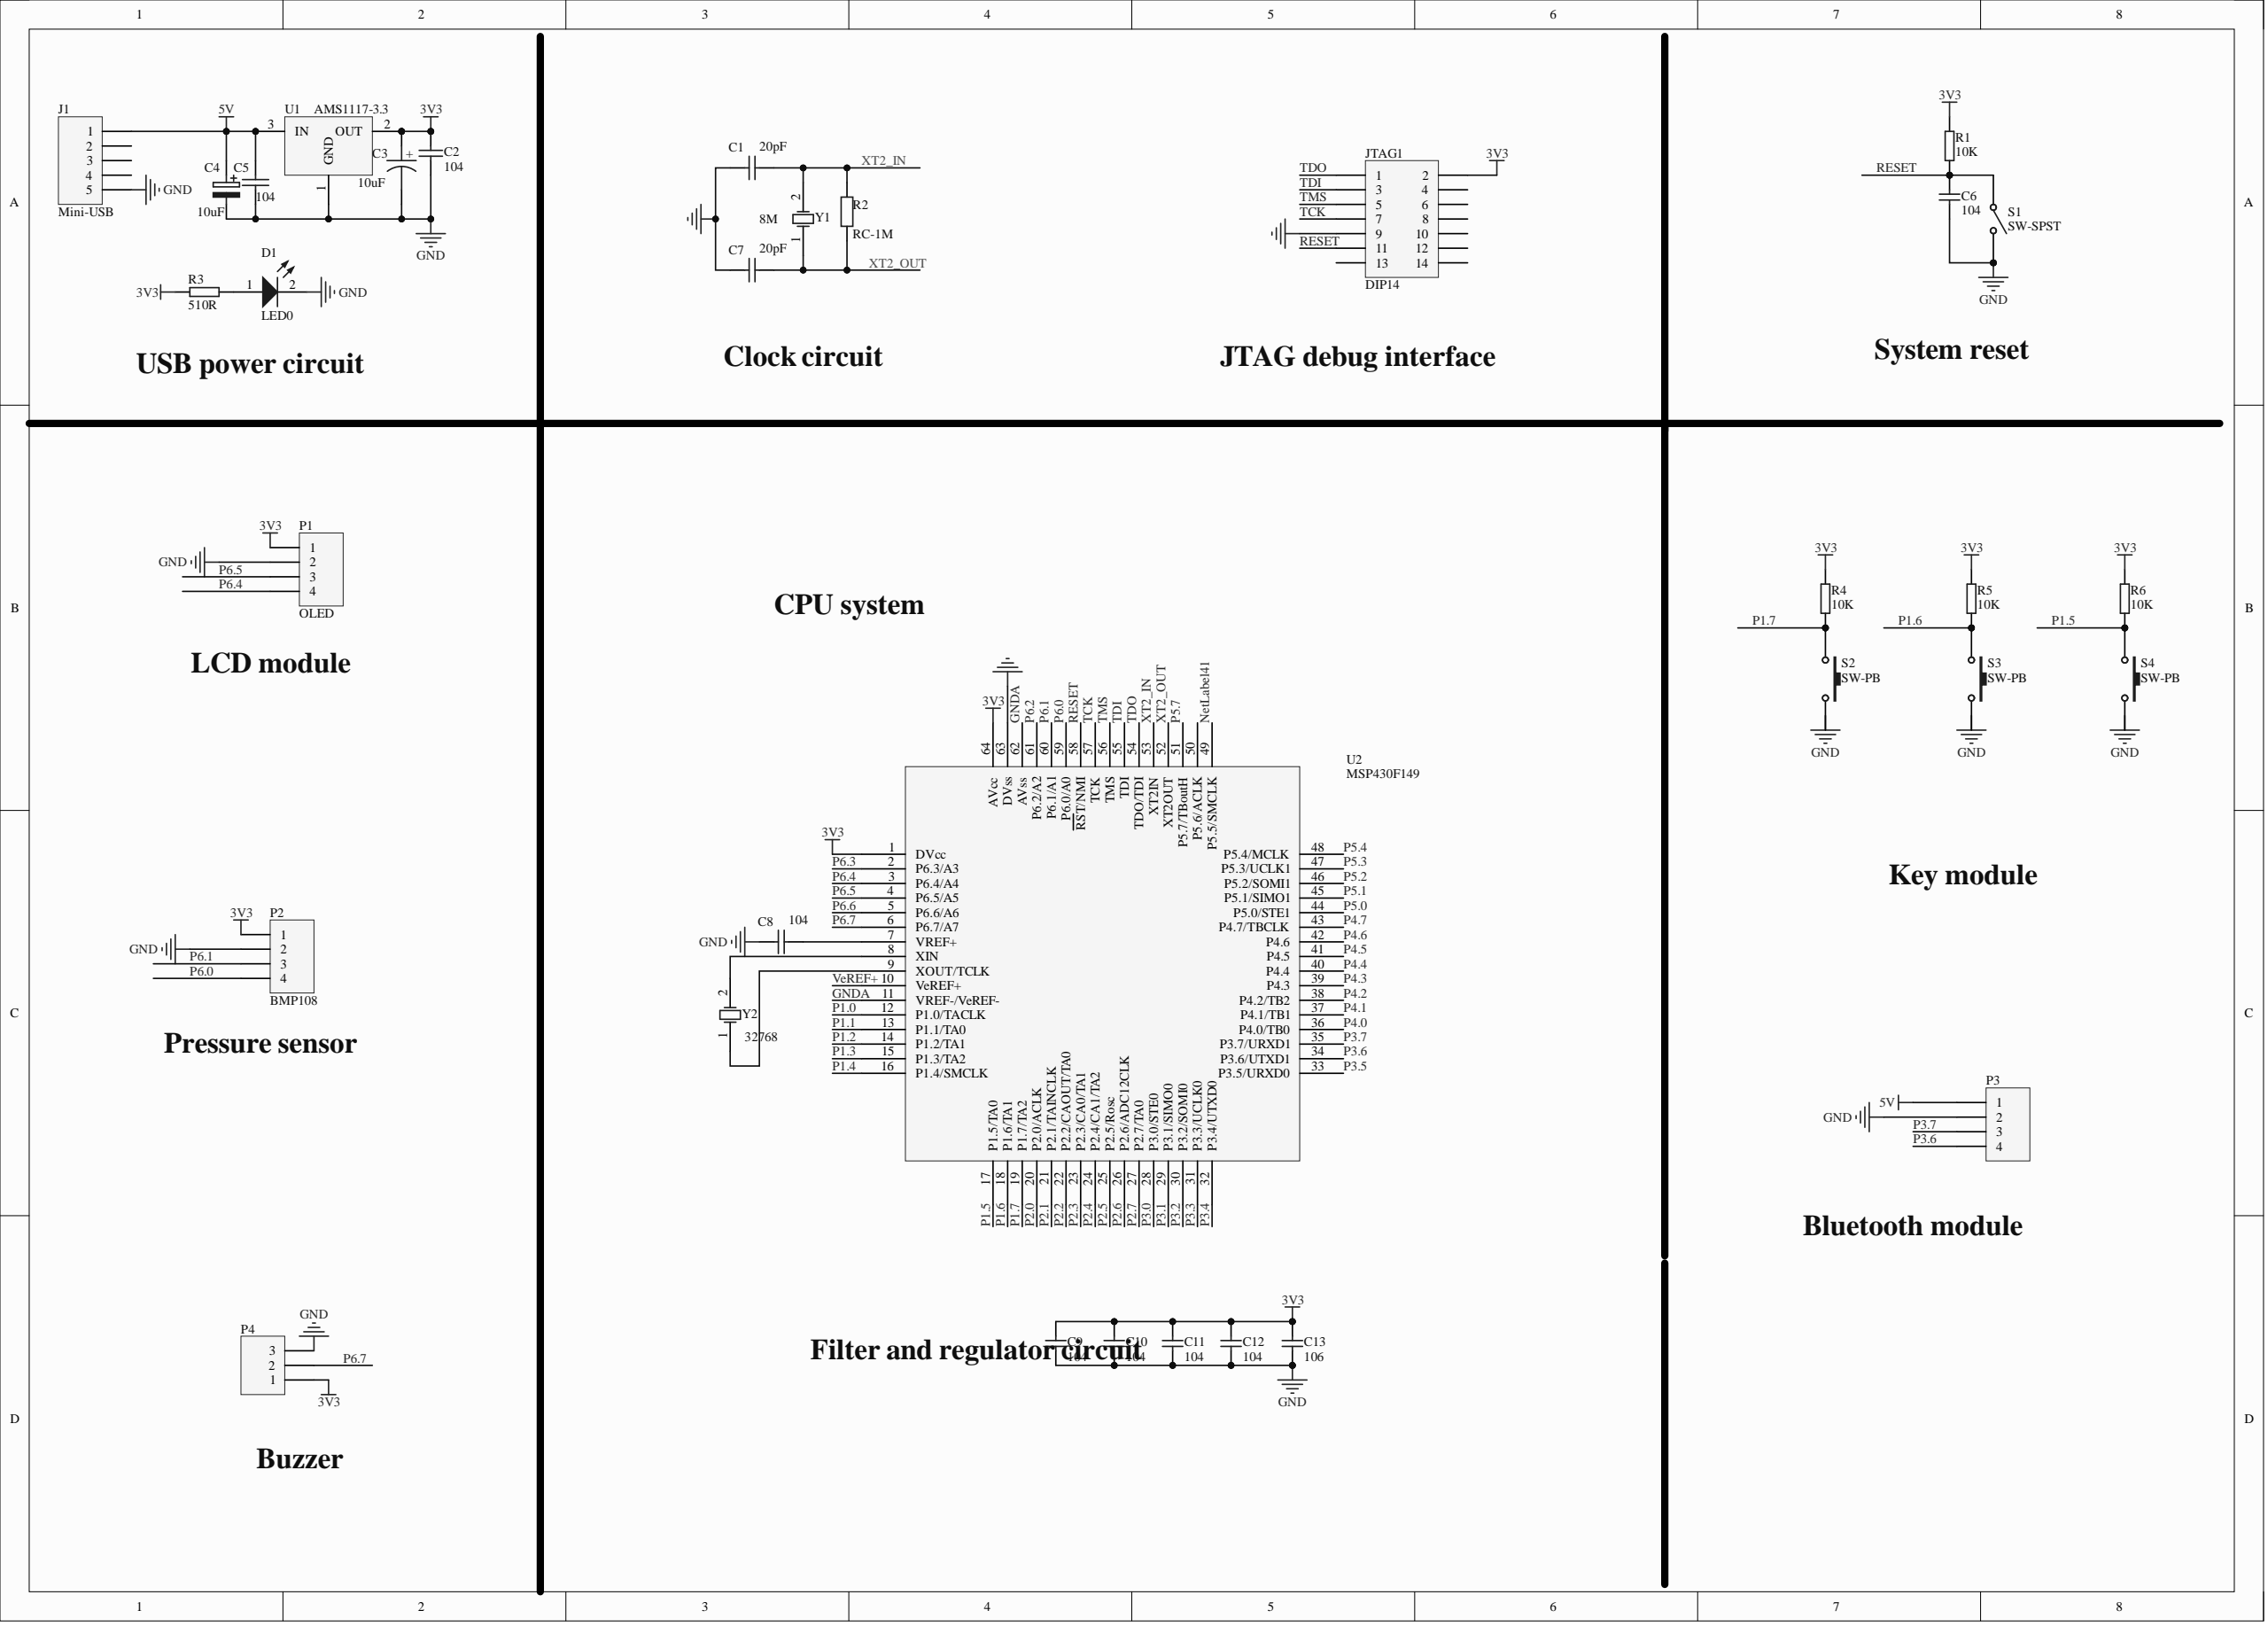Circuit board | Altium Designer | 34 parts | 25 nets
Bill of materials:
Comment,Description,Designator,Footprint,LibRef,Quantity
"S0805-20P","Capacitor","C1, C7, C8","0805C","Cap","3"
"104","Capacitor","C2, C5, C6, C9, C10, C11, C12","0603C","Cap, CAP1","7"
"10uF","Capacitor","C3","贴片电容","CAPACITOR POL","1"
"10uF","","C4","0805C","ELECTRO2","1"
"106","Capacitor","C13","0805C","CAP1","1"
"LED0","Typical INFRARED GaAs LED","D1","LED0603-RD","LED0","1"
"Mini-USB","Header, 5-Pin","J1","USB-MINI-A","Header 5","1"
"DIP14","Connectors","JTAG1","HDR2X7","DIP14","1"
"OLED","Header, 4-Pin, Right Angle","P1","HDR1X4H","Header 4H","1"
"BMP108","Header, 4-Pin, Right Angle","P2","HDR1X4H","Header 4H","1"
"Bluetooth module","Header, 4-Pin","P3","HDR1X4","Header 4","1"
"Buzzer","Header, 3-Pin","P4","HDR1X3","Header 3","1"
"10K","","R1, R4, R5, R6","0603R","R","4"
"RC-1M","Resistor","R2","0805R","Res2","1"
"510R","","R3","0603R","R","1"
"SW-SPST","Single-Pole, Single-Throw Switch","S1","SPST-2","SW-SPST","1"
"SW-PB","Switch","S2, S3, S4","SPST-2","SW-PB","3"
"AMS1117-3.3","","U1","AMS1117-3.3","LT1085CM-3.3","1"
"MSP430F149","MCU","U2","MSP430F149","MSP430F149","1"
"8M","Crystal Oscillator","Y1","XTAL-SMD-NX3215SA-32.768K-STD-MUS-2","XTAL","1"
"32768","Crystal Oscillator","Y2","XTAL-SMD-NX3215SA-32.768K-STD-MUS-2","XTAL","1"
Netlist (Protel format):
[
C1
0805C
S0805-20P



]
[
C2
0603C
104



]
[
C3
贴片电容
10uF



]
[
C4
0805C
10uF



]
[
C5
0603C
104



]
[
C6
0603C
104



]
[
C7
0805C
S0805-20P



]
[
C8
0805C
S0805-20P



]
[
C9
0603C
104



]
[
C10
0603C
104



]
[
C11
0603C
104



]
[
C12
0603C
104



]
[
C13
0805C
106



]
[
D1
LED0603-RD
LED0



]
[
J1
USB-MINI-A
Mini-USB



]
[
JTAG1
HDR2X7
DIP14



]
[
P1
HDR1X4H
OLED



]
[
P2
HDR1X4H
BMP108



]
[
P3
HDR1X4
Bluetooth module



]
[
P4
HDR1X3
Buzzer



]
[
R1
0603R
10K



]
[
R2
0805R
RC-1M



]
[
R3
0603R
510R



]
[
R4
0603R
10K



]
[
R5
0603R
10K



]
[
R6
0603R
10K



]
[
S1
SPST-2
SW-SPST



]
[
S2
SPST-2
SW-PB



]
[
S3
SPST-2
SW-PB



]
[
S4
SPST-2
SW-PB



]
[
U1
AMS1117-3.3
AMS1117-3.3



]
[
U2
MSP430F149
MSP430F149



]
[
Y1
XTAL-SMD-NX3215SA-32.768K-STD-MUS-2
8M



]
[
Y2
XTAL-SMD-NX3215SA-32.768K-STD-MUS-2
32768



]
(
XT2_OUT
C7-2
R2-1
U2-52
Y1-1
)
(
XT2_IN
C1-2
R2-2
U2-53
Y1-2
)
(
TMS
JTAG1-5
U2-56
)
(
TDO
JTAG1-1
U2-54
)
(
TDI
JTAG1-3
U2-55
)
(
TCK
JTAG1-7
U2-57
)
(
RESET
C6-1
JTAG1-11
R1-1
S1-1
U2-58
)
(
P6.7
P4-2
U2-6
)
(
P6.5
P1-3
U2-4
)
(
P6.4
P1-4
U2-3
)
(
P6.1
P2-3
U2-60
)
(
P6.0
P2-4
U2-59
)
(
P3.7
P3-3
U2-35
)
(
P3.6
P3-4
U2-34
)
(
P1.7
R4-1
S2-1
U2-19
)
(
P1.6
R5-1
S3-1
U2-18
)
(
P1.5
R6-1
S4-1
U2-17
)
(
NetU2_9
U2-9
Y2-1
)
(
NetU2_8
U2-8
Y2-2
)
(
NetD1_1
D1-1
R3-1
)
(
NetC8_2
C8-2
U2-7
)
(
GNDA
U2-11
U2-62
)
(
GND
C1-1
C2-2
C3-2
C4-2
C5-2
C6-2
C7-1
C8-1
C9-2
C10-2
C11-2
C12-2
C13-2
D1-2
J1-5
JTAG1-9
P1-2
P2-2
P3-2
P4-3
S1-2
U1-1
U2-63
)
(
5V
C4-1
C5-1
J1-1
P3-1
U1-3
)
(
3V3
C2-1
C3-1
C9-1
C10-1
C11-1
C12-1
C13-1
JTAG1-2
P1-1
P2-1
P4-1
R1-2
R3-2
R4-2
R5-2
R6-2
U1-2
U2-1
U2-64
)